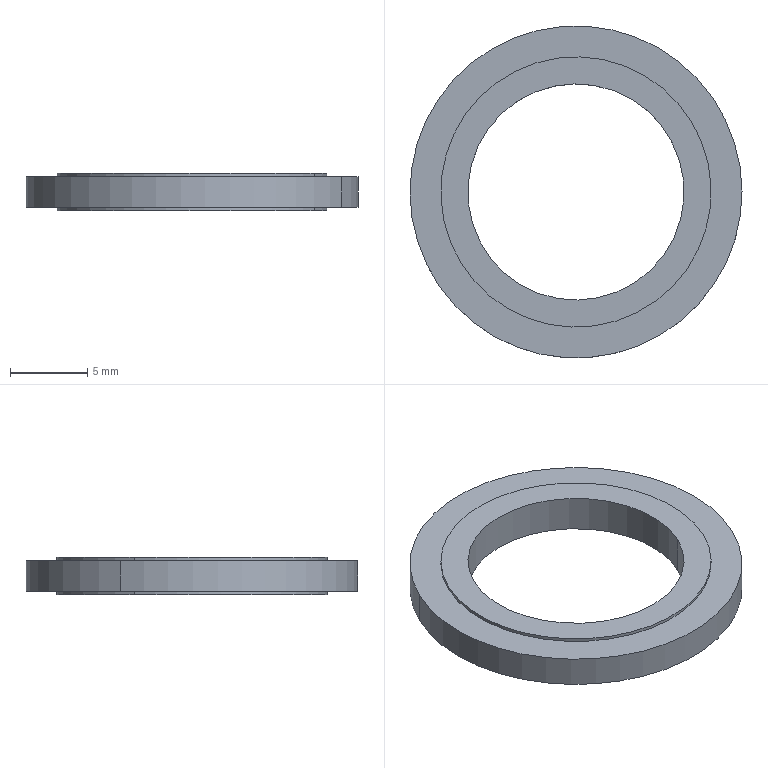Part | SolidWorks | features BaseBody 1 | 1 solid | 12 faces | box 21.5 x 21.5 x 2.4 mm | volume 452.861 mm3 | cylinder 8 | plane 4 | commonest cylinder face diameters 17.5 x4 14 x2 21.5 x2
STEP:
#1=CARTESIAN_POINT('',(214.595,128.251,100.5));
#2=VERTEX_POINT('',#1);
#3=CARTESIAN_POINT('',(230.405,120.749,100.5));
#4=VERTEX_POINT('',#3);
#5=CARTESIAN_POINT('',(222.5,124.5,100.5));
#6=DIRECTION('',(0.,0.,-1.));
#7=DIRECTION('',(-0.9034,0.4287,0.));
#8=AXIS2_PLACEMENT_3D('',#5,#6,#7);
#9=CIRCLE('',#8,8.75);
#10=EDGE_CURVE('',#2,#4,#9,.T.);
#11=ORIENTED_EDGE('',*,*,#10,.T.);
#12=CARTESIAN_POINT('',(230.405,120.749,100.3));
#13=VERTEX_POINT('',#12);
#14=CARTESIAN_POINT('',(230.405,120.749,73.582));
#15=DIRECTION('',(0.,0.,-1.));
#16=VECTOR('',#15,1000.);
#17=LINE('',#14,#16);
#18=EDGE_CURVE('',#4,#13,#17,.T.);
#19=ORIENTED_EDGE('',*,*,#18,.T.);
#20=CARTESIAN_POINT('',(214.595,128.251,100.3));
#21=VERTEX_POINT('',#20);
#22=CARTESIAN_POINT('',(222.5,124.5,100.3));
#23=DIRECTION('',(0.,0.,-1.));
#24=DIRECTION('',(-0.9034,0.4287,0.));
#25=AXIS2_PLACEMENT_3D('',#22,#23,#24);
#26=CIRCLE('',#25,8.75);
#27=EDGE_CURVE('',#21,#13,#26,.T.);
#28=ORIENTED_EDGE('',*,*,#27,.F.);
#29=CARTESIAN_POINT('',(214.595,128.251,73.582));
#30=DIRECTION('',(0.,0.,-1.));
#31=VECTOR('',#30,1000.);
#32=LINE('',#29,#31);
#33=EDGE_CURVE('',#2,#21,#32,.T.);
#34=ORIENTED_EDGE('',*,*,#33,.F.);
#35=EDGE_LOOP('',(#11,#19,#28,#34));
#36=FACE_OUTER_BOUND('',#35,.T.);
#37=CARTESIAN_POINT('',(222.5,124.5,73.582));
#38=DIRECTION('',(0.,0.,-1.));
#39=DIRECTION('',(-0.9034,0.4287,0.));
#40=AXIS2_PLACEMENT_3D('',#37,#38,#39);
#41=CYLINDRICAL_SURFACE('',#40,8.75);
#42=ADVANCED_FACE('',(#36),#41,.T.);
#43=CARTESIAN_POINT('',(228.824,121.499,102.7));
#44=VERTEX_POINT('',#43);
#45=CARTESIAN_POINT('',(216.176,127.501,102.7));
#46=VERTEX_POINT('',#45);
#47=CARTESIAN_POINT('',(222.5,124.5,102.7));
#48=DIRECTION('',(0.,0.,-1.));
#49=DIRECTION('',(-0.9034,0.4287,0.));
#50=AXIS2_PLACEMENT_3D('',#47,#48,#49);
#51=CIRCLE('',#50,7.);
#52=EDGE_CURVE('',#44,#46,#51,.T.);
#53=ORIENTED_EDGE('',*,*,#52,.F.);
#54=CARTESIAN_POINT('',(228.824,121.499,100.3));
#55=VERTEX_POINT('',#54);
#56=CARTESIAN_POINT('',(228.824,121.499,73.582));
#57=DIRECTION('',(0.,0.,-1.));
#58=VECTOR('',#57,1000.);
#59=LINE('',#56,#58);
#60=EDGE_CURVE('',#44,#55,#59,.T.);
#61=ORIENTED_EDGE('',*,*,#60,.T.);
#62=CARTESIAN_POINT('',(216.176,127.501,100.3));
#63=VERTEX_POINT('',#62);
#64=CARTESIAN_POINT('',(222.5,124.5,100.3));
#65=DIRECTION('',(0.,0.,-1.));
#66=DIRECTION('',(-0.9034,0.4287,0.));
#67=AXIS2_PLACEMENT_3D('',#64,#65,#66);
#68=CIRCLE('',#67,7.);
#69=EDGE_CURVE('',#55,#63,#68,.T.);
#70=ORIENTED_EDGE('',*,*,#69,.T.);
#71=CARTESIAN_POINT('',(216.176,127.501,73.582));
#72=DIRECTION('',(0.,0.,-1.));
#73=VECTOR('',#72,1000.);
#74=LINE('',#71,#73);
#75=EDGE_CURVE('',#46,#63,#74,.T.);
#76=ORIENTED_EDGE('',*,*,#75,.F.);
#77=EDGE_LOOP('',(#53,#61,#70,#76));
#78=FACE_OUTER_BOUND('',#77,.T.);
#79=CARTESIAN_POINT('',(222.5,124.5,73.582));
#80=DIRECTION('',(0.,0.,-1.));
#81=DIRECTION('',(-0.9034,0.4287,0.));
#82=AXIS2_PLACEMENT_3D('',#79,#80,#81);
#83=CYLINDRICAL_SURFACE('',#82,7.);
#84=ADVANCED_FACE('',(#78),#83,.F.);
#85=CARTESIAN_POINT('',(214.595,128.251,102.7));
#86=VERTEX_POINT('',#85);
#87=CARTESIAN_POINT('',(230.405,120.749,102.7));
#88=VERTEX_POINT('',#87);
#89=CARTESIAN_POINT('',(222.5,124.5,102.7));
#90=DIRECTION('',(0.,0.,-1.));
#91=DIRECTION('',(-0.9034,0.4287,0.));
#92=AXIS2_PLACEMENT_3D('',#89,#90,#91);
#93=CIRCLE('',#92,8.75);
#94=EDGE_CURVE('',#86,#88,#93,.T.);
#95=ORIENTED_EDGE('',*,*,#94,.T.);
#96=CARTESIAN_POINT('',(230.405,120.749,102.5));
#97=VERTEX_POINT('',#96);
#98=CARTESIAN_POINT('',(230.405,120.749,73.582));
#99=DIRECTION('',(0.,0.,-1.));
#100=VECTOR('',#99,1000.);
#101=LINE('',#98,#100);
#102=EDGE_CURVE('',#88,#97,#101,.T.);
#103=ORIENTED_EDGE('',*,*,#102,.T.);
#104=CARTESIAN_POINT('',(214.595,128.251,102.5));
#105=VERTEX_POINT('',#104);
#106=CARTESIAN_POINT('',(222.5,124.5,102.5));
#107=DIRECTION('',(0.,0.,-1.));
#108=DIRECTION('',(-0.9034,0.4287,0.));
#109=AXIS2_PLACEMENT_3D('',#106,#107,#108);
#110=CIRCLE('',#109,8.75);
#111=EDGE_CURVE('',#105,#97,#110,.T.);
#112=ORIENTED_EDGE('',*,*,#111,.F.);
#113=CARTESIAN_POINT('',(214.595,128.251,73.582));
#114=DIRECTION('',(0.,0.,-1.));
#115=VECTOR('',#114,1000.);
#116=LINE('',#113,#115);
#117=EDGE_CURVE('',#86,#105,#116,.T.);
#118=ORIENTED_EDGE('',*,*,#117,.F.);
#119=EDGE_LOOP('',(#95,#103,#112,#118));
#120=FACE_OUTER_BOUND('',#119,.T.);
#121=CARTESIAN_POINT('',(222.5,124.5,73.582));
#122=DIRECTION('',(0.,0.,-1.));
#123=DIRECTION('',(-0.9034,0.4287,0.));
#124=AXIS2_PLACEMENT_3D('',#121,#122,#123);
#125=CYLINDRICAL_SURFACE('',#124,8.75);
#126=ADVANCED_FACE('',(#120),#125,.T.);
#127=CARTESIAN_POINT('',(212.788,129.109,102.5));
#128=VERTEX_POINT('',#127);
#129=CARTESIAN_POINT('',(232.212,119.891,102.5));
#130=VERTEX_POINT('',#129);
#131=CARTESIAN_POINT('',(222.5,124.5,102.5));
#132=DIRECTION('',(0.,0.,-1.));
#133=DIRECTION('',(-0.9034,0.4287,0.));
#134=AXIS2_PLACEMENT_3D('',#131,#132,#133);
#135=CIRCLE('',#134,10.75);
#136=EDGE_CURVE('',#128,#130,#135,.T.);
#137=ORIENTED_EDGE('',*,*,#136,.T.);
#138=CARTESIAN_POINT('',(232.212,119.891,100.5));
#139=VERTEX_POINT('',#138);
#140=CARTESIAN_POINT('',(232.212,119.891,73.582));
#141=DIRECTION('',(0.,0.,-1.));
#142=VECTOR('',#141,1000.);
#143=LINE('',#140,#142);
#144=EDGE_CURVE('',#130,#139,#143,.T.);
#145=ORIENTED_EDGE('',*,*,#144,.T.);
#146=CARTESIAN_POINT('',(212.788,129.109,100.5));
#147=VERTEX_POINT('',#146);
#148=CARTESIAN_POINT('',(222.5,124.5,100.5));
#149=DIRECTION('',(0.,0.,-1.));
#150=DIRECTION('',(-0.9034,0.4287,0.));
#151=AXIS2_PLACEMENT_3D('',#148,#149,#150);
#152=CIRCLE('',#151,10.75);
#153=EDGE_CURVE('',#147,#139,#152,.T.);
#154=ORIENTED_EDGE('',*,*,#153,.F.);
#155=CARTESIAN_POINT('',(212.788,129.109,73.582));
#156=DIRECTION('',(0.,0.,-1.));
#157=VECTOR('',#156,1000.);
#158=LINE('',#155,#157);
#159=EDGE_CURVE('',#128,#147,#158,.T.);
#160=ORIENTED_EDGE('',*,*,#159,.F.);
#161=EDGE_LOOP('',(#137,#145,#154,#160));
#162=FACE_OUTER_BOUND('',#161,.T.);
#163=CARTESIAN_POINT('',(222.5,124.5,73.582));
#164=DIRECTION('',(0.,0.,-1.));
#165=DIRECTION('',(-0.9034,0.4287,0.));
#166=AXIS2_PLACEMENT_3D('',#163,#164,#165);
#167=CYLINDRICAL_SURFACE('',#166,10.75);
#168=ADVANCED_FACE('',(#162),#167,.T.);
#169=ORIENTED_EDGE('',*,*,#153,.T.);
#170=CARTESIAN_POINT('',(222.5,124.5,100.5));
#171=DIRECTION('',(0.,0.,-1.));
#172=DIRECTION('',(-0.9034,0.4287,0.));
#173=AXIS2_PLACEMENT_3D('',#170,#171,#172);
#174=CIRCLE('',#173,10.75);
#175=EDGE_CURVE('',#139,#147,#174,.T.);
#176=ORIENTED_EDGE('',*,*,#175,.T.);
#177=EDGE_LOOP('',(#169,#176));
#178=FACE_OUTER_BOUND('',#177,.T.);
#179=ORIENTED_EDGE('',*,*,#10,.F.);
#180=CARTESIAN_POINT('',(222.5,124.5,100.5));
#181=DIRECTION('',(0.,0.,-1.));
#182=DIRECTION('',(-0.9034,0.4287,0.));
#183=AXIS2_PLACEMENT_3D('',#180,#181,#182);
#184=CIRCLE('',#183,8.75);
#185=EDGE_CURVE('',#4,#2,#184,.T.);
#186=ORIENTED_EDGE('',*,*,#185,.F.);
#187=EDGE_LOOP('',(#179,#186));
#188=FACE_BOUND('',#187,.T.);
#189=CARTESIAN_POINT('',(217.891,114.788,100.5));
#190=DIRECTION('',(0.,0.,-1.));
#191=DIRECTION('',(-0.9034,0.4287,0.));
#192=AXIS2_PLACEMENT_3D('',#189,#190,#191);
#193=PLANE('',#192);
#194=ADVANCED_FACE('',(#178,#188),#193,.T.);
#195=ORIENTED_EDGE('',*,*,#144,.F.);
#196=CARTESIAN_POINT('',(222.5,124.5,102.5));
#197=DIRECTION('',(0.,0.,-1.));
#198=DIRECTION('',(-0.9034,0.4287,0.));
#199=AXIS2_PLACEMENT_3D('',#196,#197,#198);
#200=CIRCLE('',#199,10.75);
#201=EDGE_CURVE('',#130,#128,#200,.T.);
#202=ORIENTED_EDGE('',*,*,#201,.T.);
#203=ORIENTED_EDGE('',*,*,#159,.T.);
#204=ORIENTED_EDGE('',*,*,#175,.F.);
#205=EDGE_LOOP('',(#195,#202,#203,#204));
#206=FACE_OUTER_BOUND('',#205,.T.);
#207=CARTESIAN_POINT('',(222.5,124.5,73.582));
#208=DIRECTION('',(0.,0.,-1.));
#209=DIRECTION('',(-0.9034,0.4287,0.));
#210=AXIS2_PLACEMENT_3D('',#207,#208,#209);
#211=CYLINDRICAL_SURFACE('',#210,10.75);
#212=ADVANCED_FACE('',(#206),#211,.T.);
#213=ORIENTED_EDGE('',*,*,#111,.T.);
#214=CARTESIAN_POINT('',(222.5,124.5,102.5));
#215=DIRECTION('',(0.,0.,-1.));
#216=DIRECTION('',(-0.9034,0.4287,0.));
#217=AXIS2_PLACEMENT_3D('',#214,#215,#216);
#218=CIRCLE('',#217,8.75);
#219=EDGE_CURVE('',#97,#105,#218,.T.);
#220=ORIENTED_EDGE('',*,*,#219,.T.);
#221=EDGE_LOOP('',(#213,#220));
#222=FACE_BOUND('',#221,.T.);
#223=ORIENTED_EDGE('',*,*,#136,.F.);
#224=ORIENTED_EDGE('',*,*,#201,.F.);
#225=EDGE_LOOP('',(#223,#224));
#226=FACE_OUTER_BOUND('',#225,.T.);
#227=CARTESIAN_POINT('',(217.891,114.788,102.5));
#228=DIRECTION('',(0.,0.,1.));
#229=DIRECTION('',(0.9034,-0.4287,0.));
#230=AXIS2_PLACEMENT_3D('',#227,#228,#229);
#231=PLANE('',#230);
#232=ADVANCED_FACE('',(#222,#226),#231,.T.);
#233=ORIENTED_EDGE('',*,*,#102,.F.);
#234=CARTESIAN_POINT('',(222.5,124.5,102.7));
#235=DIRECTION('',(0.,0.,-1.));
#236=DIRECTION('',(-0.9034,0.4287,0.));
#237=AXIS2_PLACEMENT_3D('',#234,#235,#236);
#238=CIRCLE('',#237,8.75);
#239=EDGE_CURVE('',#88,#86,#238,.T.);
#240=ORIENTED_EDGE('',*,*,#239,.T.);
#241=ORIENTED_EDGE('',*,*,#117,.T.);
#242=ORIENTED_EDGE('',*,*,#219,.F.);
#243=EDGE_LOOP('',(#233,#240,#241,#242));
#244=FACE_OUTER_BOUND('',#243,.T.);
#245=CARTESIAN_POINT('',(222.5,124.5,73.582));
#246=DIRECTION('',(0.,0.,-1.));
#247=DIRECTION('',(-0.9034,0.4287,0.));
#248=AXIS2_PLACEMENT_3D('',#245,#246,#247);
#249=CYLINDRICAL_SURFACE('',#248,8.75);
#250=ADVANCED_FACE('',(#244),#249,.T.);
#251=CARTESIAN_POINT('',(222.5,124.5,102.7));
#252=DIRECTION('',(0.,0.,-1.));
#253=DIRECTION('',(-0.9034,0.4287,0.));
#254=AXIS2_PLACEMENT_3D('',#251,#252,#253);
#255=CIRCLE('',#254,7.);
#256=EDGE_CURVE('',#46,#44,#255,.T.);
#257=ORIENTED_EDGE('',*,*,#256,.T.);
#258=ORIENTED_EDGE('',*,*,#52,.T.);
#259=EDGE_LOOP('',(#257,#258));
#260=FACE_BOUND('',#259,.T.);
#261=ORIENTED_EDGE('',*,*,#94,.F.);
#262=ORIENTED_EDGE('',*,*,#239,.F.);
#263=EDGE_LOOP('',(#261,#262));
#264=FACE_OUTER_BOUND('',#263,.T.);
#265=CARTESIAN_POINT('',(218.749,116.595,102.7));
#266=DIRECTION('',(0.,0.,1.));
#267=DIRECTION('',(0.9034,-0.4287,0.));
#268=AXIS2_PLACEMENT_3D('',#265,#266,#267);
#269=PLANE('',#268);
#270=ADVANCED_FACE('',(#260,#264),#269,.T.);
#271=ORIENTED_EDGE('',*,*,#60,.F.);
#272=ORIENTED_EDGE('',*,*,#256,.F.);
#273=ORIENTED_EDGE('',*,*,#75,.T.);
#274=CARTESIAN_POINT('',(222.5,124.5,100.3));
#275=DIRECTION('',(0.,0.,-1.));
#276=DIRECTION('',(-0.9034,0.4287,0.));
#277=AXIS2_PLACEMENT_3D('',#274,#275,#276);
#278=CIRCLE('',#277,7.);
#279=EDGE_CURVE('',#63,#55,#278,.T.);
#280=ORIENTED_EDGE('',*,*,#279,.T.);
#281=EDGE_LOOP('',(#271,#272,#273,#280));
#282=FACE_OUTER_BOUND('',#281,.T.);
#283=CARTESIAN_POINT('',(222.5,124.5,73.582));
#284=DIRECTION('',(0.,0.,-1.));
#285=DIRECTION('',(-0.9034,0.4287,0.));
#286=AXIS2_PLACEMENT_3D('',#283,#284,#285);
#287=CYLINDRICAL_SURFACE('',#286,7.);
#288=ADVANCED_FACE('',(#282),#287,.F.);
#289=ORIENTED_EDGE('',*,*,#27,.T.);
#290=CARTESIAN_POINT('',(222.5,124.5,100.3));
#291=DIRECTION('',(0.,0.,-1.));
#292=DIRECTION('',(-0.9034,0.4287,0.));
#293=AXIS2_PLACEMENT_3D('',#290,#291,#292);
#294=CIRCLE('',#293,8.75);
#295=EDGE_CURVE('',#13,#21,#294,.T.);
#296=ORIENTED_EDGE('',*,*,#295,.T.);
#297=EDGE_LOOP('',(#289,#296));
#298=FACE_OUTER_BOUND('',#297,.T.);
#299=ORIENTED_EDGE('',*,*,#279,.F.);
#300=ORIENTED_EDGE('',*,*,#69,.F.);
#301=EDGE_LOOP('',(#299,#300));
#302=FACE_BOUND('',#301,.T.);
#303=CARTESIAN_POINT('',(218.749,116.595,100.3));
#304=DIRECTION('',(0.,0.,-1.));
#305=DIRECTION('',(-0.9034,0.4287,0.));
#306=AXIS2_PLACEMENT_3D('',#303,#304,#305);
#307=PLANE('',#306);
#308=ADVANCED_FACE('',(#298,#302),#307,.T.);
#309=ORIENTED_EDGE('',*,*,#18,.F.);
#310=ORIENTED_EDGE('',*,*,#185,.T.);
#311=ORIENTED_EDGE('',*,*,#33,.T.);
#312=ORIENTED_EDGE('',*,*,#295,.F.);
#313=EDGE_LOOP('',(#309,#310,#311,#312));
#314=FACE_OUTER_BOUND('',#313,.T.);
#315=CARTESIAN_POINT('',(222.5,124.5,73.582));
#316=DIRECTION('',(0.,0.,-1.));
#317=DIRECTION('',(-0.9034,0.4287,0.));
#318=AXIS2_PLACEMENT_3D('',#315,#316,#317);
#319=CYLINDRICAL_SURFACE('',#318,8.75);
#320=ADVANCED_FACE('',(#314),#319,.T.);
#321=CLOSED_SHELL('',(#42,#84,#126,#168,#194,#212,#232,#250,#270,#288,#308,#320));
#322=MANIFOLD_SOLID_BREP('',#321);
#323=CARTESIAN_POINT('',(0.,0.,0.));
#324=DIRECTION('',(0.,0.,1.));
#325=DIRECTION('',(1.,0.,0.));
#326=AXIS2_PLACEMENT_3D('',#323,#324,#325);
#327=(LENGTH_UNIT()NAMED_UNIT(*)SI_UNIT(.MILLI.,.METRE.));
#328=UNCERTAINTY_MEASURE_WITH_UNIT(LENGTH_MEASURE(0.00001),#327,'','');
#329=(NAMED_UNIT(*)PLANE_ANGLE_UNIT()SI_UNIT($,.RADIAN.));
#330=(NAMED_UNIT(*)SI_UNIT($,.STERADIAN.)SOLID_ANGLE_UNIT());
#331=(GEOMETRIC_REPRESENTATION_CONTEXT(3)GLOBAL_UNCERTAINTY_ASSIGNED_CONTEXT((#328))GLOBAL_UNIT_ASSIGNED_CONTEXT((#327,#329,#330))REPRESENTATION_CONTEXT('',''));
#332=ADVANCED_BREP_SHAPE_REPRESENTATION('',(#322,#326),#331);